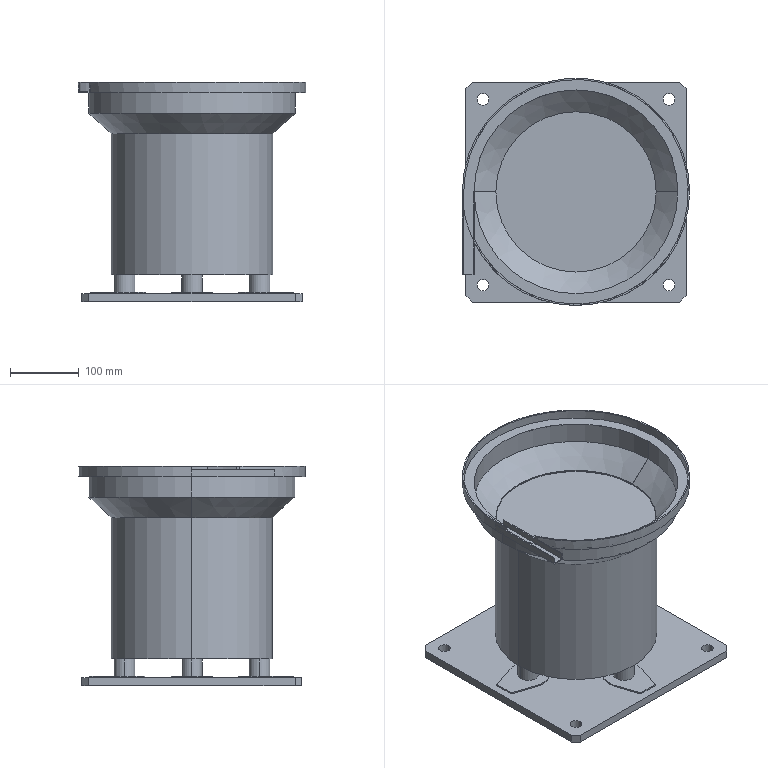Part | STEP file | Mount electronic clip vibrating plate BM23-2V1 part | 1 solid | 85 faces | box 330 x 330 x 319 mm | volume 10354356 mm3 | plane 43 | cylinder 38 | cone 4 | commonest cylinder face diameters 60 x9 17 x8 30 x8 330 x4 232.847 x2 234.4 x2